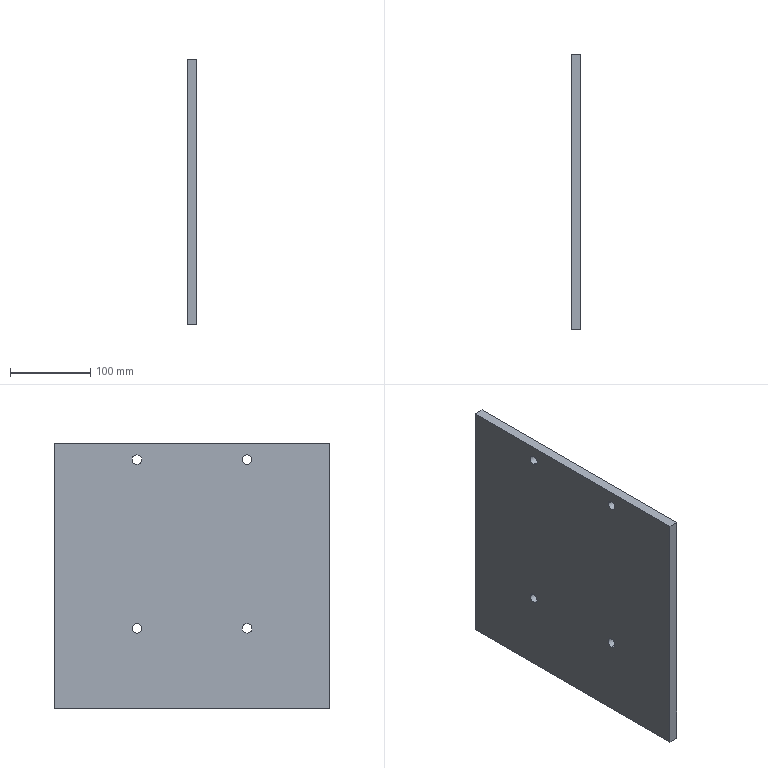Part | SolidWorks | features BaseBody 1 | 1 solid | 14 faces | box 12 x 344.147 x 330 mm | volume 1357393 mm3 | cylinder 8 | plane 6 | commonest cylinder face diameters 12 x8
STEP:
#1=CARTESIAN_POINT('',(-546.442,569.924,584.465));
#2=VERTEX_POINT('',#1);
#3=CARTESIAN_POINT('',(-546.442,569.924,596.465));
#4=VERTEX_POINT('',#3);
#5=CARTESIAN_POINT('',(-546.442,569.924,590.465));
#6=DIRECTION('',(-1.,0.,0.));
#7=DIRECTION('',(0.,0.,1.));
#8=AXIS2_PLACEMENT_3D('',#5,#6,#7);
#9=CIRCLE('',#8,6.);
#10=EDGE_CURVE('',#2,#4,#9,.T.);
#11=ORIENTED_EDGE('',*,*,#10,.T.);
#12=CARTESIAN_POINT('',(-534.442,569.924,596.465));
#13=VERTEX_POINT('',#12);
#14=CARTESIAN_POINT('',(-619.405,569.924,596.465));
#15=DIRECTION('',(1.,0.,0.));
#16=VECTOR('',#15,1000.);
#17=LINE('',#14,#16);
#18=EDGE_CURVE('',#4,#13,#17,.T.);
#19=ORIENTED_EDGE('',*,*,#18,.T.);
#20=CARTESIAN_POINT('',(-534.442,569.924,584.465));
#21=VERTEX_POINT('',#20);
#22=CARTESIAN_POINT('',(-534.442,569.924,590.465));
#23=DIRECTION('',(-1.,0.,0.));
#24=DIRECTION('',(0.,0.,1.));
#25=AXIS2_PLACEMENT_3D('',#22,#23,#24);
#26=CIRCLE('',#25,6.);
#27=EDGE_CURVE('',#21,#13,#26,.T.);
#28=ORIENTED_EDGE('',*,*,#27,.F.);
#29=CARTESIAN_POINT('',(-619.405,569.924,584.465));
#30=DIRECTION('',(1.,0.,0.));
#31=VECTOR('',#30,1000.);
#32=LINE('',#29,#31);
#33=EDGE_CURVE('',#2,#21,#32,.T.);
#34=ORIENTED_EDGE('',*,*,#33,.F.);
#35=EDGE_LOOP('',(#11,#19,#28,#34));
#36=FACE_OUTER_BOUND('',#35,.T.);
#37=CARTESIAN_POINT('',(-619.405,569.924,590.465));
#38=DIRECTION('',(1.,0.,0.));
#39=DIRECTION('',(0.,0.,-1.));
#40=AXIS2_PLACEMENT_3D('',#37,#38,#39);
#41=CYLINDRICAL_SURFACE('',#40,6.);
#42=ADVANCED_FACE('',(#36),#41,.F.);
#43=CARTESIAN_POINT('',(-546.442,569.924,590.465));
#44=DIRECTION('',(-1.,0.,0.));
#45=DIRECTION('',(0.,0.,1.));
#46=AXIS2_PLACEMENT_3D('',#43,#44,#45);
#47=CIRCLE('',#46,6.);
#48=EDGE_CURVE('',#4,#2,#47,.T.);
#49=ORIENTED_EDGE('',*,*,#48,.T.);
#50=ORIENTED_EDGE('',*,*,#33,.T.);
#51=CARTESIAN_POINT('',(-534.442,569.924,590.465));
#52=DIRECTION('',(-1.,0.,0.));
#53=DIRECTION('',(0.,0.,1.));
#54=AXIS2_PLACEMENT_3D('',#51,#52,#53);
#55=CIRCLE('',#54,6.);
#56=EDGE_CURVE('',#13,#21,#55,.T.);
#57=ORIENTED_EDGE('',*,*,#56,.F.);
#58=ORIENTED_EDGE('',*,*,#18,.F.);
#59=EDGE_LOOP('',(#49,#50,#57,#58));
#60=FACE_OUTER_BOUND('',#59,.T.);
#61=CARTESIAN_POINT('',(-619.405,569.924,590.465));
#62=DIRECTION('',(1.,0.,0.));
#63=DIRECTION('',(0.,0.,-1.));
#64=AXIS2_PLACEMENT_3D('',#61,#62,#63);
#65=CYLINDRICAL_SURFACE('',#64,6.);
#66=ADVANCED_FACE('',(#60),#65,.F.);
#67=CARTESIAN_POINT('',(-546.442,563.924,379.749));
#68=VERTEX_POINT('',#67);
#69=CARTESIAN_POINT('',(-546.442,575.924,379.749));
#70=VERTEX_POINT('',#69);
#71=CARTESIAN_POINT('',(-546.442,569.924,379.749));
#72=DIRECTION('',(-1.,0.,0.));
#73=DIRECTION('',(0.,0.,1.));
#74=AXIS2_PLACEMENT_3D('',#71,#72,#73);
#75=CIRCLE('',#74,6.);
#76=EDGE_CURVE('',#68,#70,#75,.T.);
#77=ORIENTED_EDGE('',*,*,#76,.T.);
#78=CARTESIAN_POINT('',(-534.442,575.924,379.749));
#79=VERTEX_POINT('',#78);
#80=CARTESIAN_POINT('',(-619.405,575.924,379.749));
#81=DIRECTION('',(1.,0.,0.));
#82=VECTOR('',#81,1000.);
#83=LINE('',#80,#82);
#84=EDGE_CURVE('',#70,#79,#83,.T.);
#85=ORIENTED_EDGE('',*,*,#84,.T.);
#86=CARTESIAN_POINT('',(-534.442,563.924,379.749));
#87=VERTEX_POINT('',#86);
#88=CARTESIAN_POINT('',(-534.442,569.924,379.749));
#89=DIRECTION('',(-1.,0.,0.));
#90=DIRECTION('',(0.,0.,1.));
#91=AXIS2_PLACEMENT_3D('',#88,#89,#90);
#92=CIRCLE('',#91,6.);
#93=EDGE_CURVE('',#87,#79,#92,.T.);
#94=ORIENTED_EDGE('',*,*,#93,.F.);
#95=CARTESIAN_POINT('',(-619.405,563.924,379.749));
#96=DIRECTION('',(1.,0.,0.));
#97=VECTOR('',#96,1000.);
#98=LINE('',#95,#97);
#99=EDGE_CURVE('',#68,#87,#98,.T.);
#100=ORIENTED_EDGE('',*,*,#99,.F.);
#101=EDGE_LOOP('',(#77,#85,#94,#100));
#102=FACE_OUTER_BOUND('',#101,.T.);
#103=CARTESIAN_POINT('',(-619.405,569.924,379.749));
#104=DIRECTION('',(1.,0.,0.));
#105=DIRECTION('',(0.,-1.,0.));
#106=AXIS2_PLACEMENT_3D('',#103,#104,#105);
#107=CYLINDRICAL_SURFACE('',#106,6.);
#108=ADVANCED_FACE('',(#102),#107,.F.);
#109=CARTESIAN_POINT('',(-546.442,569.924,379.749));
#110=DIRECTION('',(-1.,0.,0.));
#111=DIRECTION('',(0.,0.,1.));
#112=AXIS2_PLACEMENT_3D('',#109,#110,#111);
#113=CIRCLE('',#112,6.);
#114=EDGE_CURVE('',#70,#68,#113,.T.);
#115=ORIENTED_EDGE('',*,*,#114,.T.);
#116=ORIENTED_EDGE('',*,*,#99,.T.);
#117=CARTESIAN_POINT('',(-534.442,569.924,379.749));
#118=DIRECTION('',(-1.,0.,0.));
#119=DIRECTION('',(0.,0.,1.));
#120=AXIS2_PLACEMENT_3D('',#117,#118,#119);
#121=CIRCLE('',#120,6.);
#122=EDGE_CURVE('',#79,#87,#121,.T.);
#123=ORIENTED_EDGE('',*,*,#122,.F.);
#124=ORIENTED_EDGE('',*,*,#84,.F.);
#125=EDGE_LOOP('',(#115,#116,#123,#124));
#126=FACE_OUTER_BOUND('',#125,.T.);
#127=CARTESIAN_POINT('',(-619.405,569.924,379.749));
#128=DIRECTION('',(1.,0.,0.));
#129=DIRECTION('',(0.,-1.,0.));
#130=AXIS2_PLACEMENT_3D('',#127,#128,#129);
#131=CYLINDRICAL_SURFACE('',#130,6.);
#132=ADVANCED_FACE('',(#126),#131,.F.);
#133=CARTESIAN_POINT('',(-546.442,432.283,373.749));
#134=VERTEX_POINT('',#133);
#135=CARTESIAN_POINT('',(-546.442,432.283,385.749));
#136=VERTEX_POINT('',#135);
#137=CARTESIAN_POINT('',(-546.442,432.283,379.749));
#138=DIRECTION('',(-1.,0.,0.));
#139=DIRECTION('',(0.,0.,1.));
#140=AXIS2_PLACEMENT_3D('',#137,#138,#139);
#141=CIRCLE('',#140,6.);
#142=EDGE_CURVE('',#134,#136,#141,.T.);
#143=ORIENTED_EDGE('',*,*,#142,.T.);
#144=CARTESIAN_POINT('',(-534.442,432.283,385.749));
#145=VERTEX_POINT('',#144);
#146=CARTESIAN_POINT('',(-619.405,432.283,385.749));
#147=DIRECTION('',(1.,0.,0.));
#148=VECTOR('',#147,1000.);
#149=LINE('',#146,#148);
#150=EDGE_CURVE('',#136,#145,#149,.T.);
#151=ORIENTED_EDGE('',*,*,#150,.T.);
#152=CARTESIAN_POINT('',(-534.442,432.283,373.749));
#153=VERTEX_POINT('',#152);
#154=CARTESIAN_POINT('',(-534.442,432.283,379.749));
#155=DIRECTION('',(-1.,0.,0.));
#156=DIRECTION('',(0.,0.,1.));
#157=AXIS2_PLACEMENT_3D('',#154,#155,#156);
#158=CIRCLE('',#157,6.);
#159=EDGE_CURVE('',#153,#145,#158,.T.);
#160=ORIENTED_EDGE('',*,*,#159,.F.);
#161=CARTESIAN_POINT('',(-619.405,432.283,373.749));
#162=DIRECTION('',(1.,0.,0.));
#163=VECTOR('',#162,1000.);
#164=LINE('',#161,#163);
#165=EDGE_CURVE('',#134,#153,#164,.T.);
#166=ORIENTED_EDGE('',*,*,#165,.F.);
#167=EDGE_LOOP('',(#143,#151,#160,#166));
#168=FACE_OUTER_BOUND('',#167,.T.);
#169=CARTESIAN_POINT('',(-619.405,432.283,379.749));
#170=DIRECTION('',(1.,0.,0.));
#171=DIRECTION('',(0.,0.,-1.));
#172=AXIS2_PLACEMENT_3D('',#169,#170,#171);
#173=CYLINDRICAL_SURFACE('',#172,6.);
#174=ADVANCED_FACE('',(#168),#173,.F.);
#175=CARTESIAN_POINT('',(-546.442,432.283,379.749));
#176=DIRECTION('',(-1.,0.,0.));
#177=DIRECTION('',(0.,0.,1.));
#178=AXIS2_PLACEMENT_3D('',#175,#176,#177);
#179=CIRCLE('',#178,6.);
#180=EDGE_CURVE('',#136,#134,#179,.T.);
#181=ORIENTED_EDGE('',*,*,#180,.T.);
#182=ORIENTED_EDGE('',*,*,#165,.T.);
#183=CARTESIAN_POINT('',(-534.442,432.283,379.749));
#184=DIRECTION('',(-1.,0.,0.));
#185=DIRECTION('',(0.,0.,1.));
#186=AXIS2_PLACEMENT_3D('',#183,#184,#185);
#187=CIRCLE('',#186,6.);
#188=EDGE_CURVE('',#145,#153,#187,.T.);
#189=ORIENTED_EDGE('',*,*,#188,.F.);
#190=ORIENTED_EDGE('',*,*,#150,.F.);
#191=EDGE_LOOP('',(#181,#182,#189,#190));
#192=FACE_OUTER_BOUND('',#191,.T.);
#193=CARTESIAN_POINT('',(-619.405,432.283,379.749));
#194=DIRECTION('',(1.,0.,0.));
#195=DIRECTION('',(0.,0.,-1.));
#196=AXIS2_PLACEMENT_3D('',#193,#194,#195);
#197=CYLINDRICAL_SURFACE('',#196,6.);
#198=ADVANCED_FACE('',(#192),#197,.F.);
#199=CARTESIAN_POINT('',(-546.442,438.283,590.465));
#200=VERTEX_POINT('',#199);
#201=CARTESIAN_POINT('',(-546.442,426.283,590.465));
#202=VERTEX_POINT('',#201);
#203=CARTESIAN_POINT('',(-546.442,432.283,590.465));
#204=DIRECTION('',(-1.,0.,0.));
#205=DIRECTION('',(0.,0.,1.));
#206=AXIS2_PLACEMENT_3D('',#203,#204,#205);
#207=CIRCLE('',#206,6.);
#208=EDGE_CURVE('',#200,#202,#207,.T.);
#209=ORIENTED_EDGE('',*,*,#208,.T.);
#210=CARTESIAN_POINT('',(-534.442,426.283,590.465));
#211=VERTEX_POINT('',#210);
#212=CARTESIAN_POINT('',(-619.405,426.283,590.465));
#213=DIRECTION('',(1.,0.,0.));
#214=VECTOR('',#213,1000.);
#215=LINE('',#212,#214);
#216=EDGE_CURVE('',#202,#211,#215,.T.);
#217=ORIENTED_EDGE('',*,*,#216,.T.);
#218=CARTESIAN_POINT('',(-534.442,438.283,590.465));
#219=VERTEX_POINT('',#218);
#220=CARTESIAN_POINT('',(-534.442,432.283,590.465));
#221=DIRECTION('',(-1.,0.,0.));
#222=DIRECTION('',(0.,0.,1.));
#223=AXIS2_PLACEMENT_3D('',#220,#221,#222);
#224=CIRCLE('',#223,6.);
#225=EDGE_CURVE('',#219,#211,#224,.T.);
#226=ORIENTED_EDGE('',*,*,#225,.F.);
#227=CARTESIAN_POINT('',(-619.405,438.283,590.465));
#228=DIRECTION('',(1.,0.,0.));
#229=VECTOR('',#228,1000.);
#230=LINE('',#227,#229);
#231=EDGE_CURVE('',#200,#219,#230,.T.);
#232=ORIENTED_EDGE('',*,*,#231,.F.);
#233=EDGE_LOOP('',(#209,#217,#226,#232));
#234=FACE_OUTER_BOUND('',#233,.T.);
#235=CARTESIAN_POINT('',(-619.405,432.283,590.465));
#236=DIRECTION('',(1.,0.,0.));
#237=DIRECTION('',(0.,1.,0.));
#238=AXIS2_PLACEMENT_3D('',#235,#236,#237);
#239=CYLINDRICAL_SURFACE('',#238,6.);
#240=ADVANCED_FACE('',(#234),#239,.F.);
#241=CARTESIAN_POINT('',(-546.442,432.283,590.465));
#242=DIRECTION('',(-1.,0.,0.));
#243=DIRECTION('',(0.,0.,1.));
#244=AXIS2_PLACEMENT_3D('',#241,#242,#243);
#245=CIRCLE('',#244,6.);
#246=EDGE_CURVE('',#202,#200,#245,.T.);
#247=ORIENTED_EDGE('',*,*,#246,.T.);
#248=ORIENTED_EDGE('',*,*,#231,.T.);
#249=CARTESIAN_POINT('',(-534.442,432.283,590.465));
#250=DIRECTION('',(-1.,0.,0.));
#251=DIRECTION('',(0.,0.,1.));
#252=AXIS2_PLACEMENT_3D('',#249,#250,#251);
#253=CIRCLE('',#252,6.);
#254=EDGE_CURVE('',#211,#219,#253,.T.);
#255=ORIENTED_EDGE('',*,*,#254,.F.);
#256=ORIENTED_EDGE('',*,*,#216,.F.);
#257=EDGE_LOOP('',(#247,#248,#255,#256));
#258=FACE_OUTER_BOUND('',#257,.T.);
#259=CARTESIAN_POINT('',(-619.405,432.283,590.465));
#260=DIRECTION('',(1.,0.,0.));
#261=DIRECTION('',(0.,1.,0.));
#262=AXIS2_PLACEMENT_3D('',#259,#260,#261);
#263=CYLINDRICAL_SURFACE('',#262,6.);
#264=ADVANCED_FACE('',(#258),#263,.F.);
#265=ORIENTED_EDGE('',*,*,#225,.T.);
#266=ORIENTED_EDGE('',*,*,#254,.T.);
#267=EDGE_LOOP('',(#265,#266));
#268=FACE_BOUND('',#267,.T.);
#269=ORIENTED_EDGE('',*,*,#159,.T.);
#270=ORIENTED_EDGE('',*,*,#188,.T.);
#271=EDGE_LOOP('',(#269,#270));
#272=FACE_BOUND('',#271,.T.);
#273=ORIENTED_EDGE('',*,*,#93,.T.);
#274=ORIENTED_EDGE('',*,*,#122,.T.);
#275=EDGE_LOOP('',(#273,#274));
#276=FACE_BOUND('',#275,.T.);
#277=ORIENTED_EDGE('',*,*,#27,.T.);
#278=ORIENTED_EDGE('',*,*,#56,.T.);
#279=EDGE_LOOP('',(#277,#278));
#280=FACE_BOUND('',#279,.T.);
#281=CARTESIAN_POINT('',(-534.442,329.03,280.107));
#282=VERTEX_POINT('',#281);
#283=CARTESIAN_POINT('',(-534.442,673.177,280.107));
#284=VERTEX_POINT('',#283);
#285=CARTESIAN_POINT('',(-534.442,409.03,280.107));
#286=DIRECTION('',(0.,1.,0.));
#287=VECTOR('',#286,1000.);
#288=LINE('',#285,#287);
#289=EDGE_CURVE('',#282,#284,#288,.T.);
#290=ORIENTED_EDGE('',*,*,#289,.T.);
#291=CARTESIAN_POINT('',(-534.442,673.177,610.107));
#292=VERTEX_POINT('',#291);
#293=CARTESIAN_POINT('',(-534.442,673.177,610.107));
#294=DIRECTION('',(0.,0.,1.));
#295=VECTOR('',#294,1000.);
#296=LINE('',#293,#295);
#297=EDGE_CURVE('',#284,#292,#296,.T.);
#298=ORIENTED_EDGE('',*,*,#297,.T.);
#299=CARTESIAN_POINT('',(-534.442,329.03,610.107));
#300=VERTEX_POINT('',#299);
#301=CARTESIAN_POINT('',(-534.442,409.03,610.107));
#302=DIRECTION('',(0.,-1.,0.));
#303=VECTOR('',#302,1000.);
#304=LINE('',#301,#303);
#305=EDGE_CURVE('',#292,#300,#304,.T.);
#306=ORIENTED_EDGE('',*,*,#305,.T.);
#307=CARTESIAN_POINT('',(-534.442,329.03,610.107));
#308=DIRECTION('',(0.,0.,-1.));
#309=VECTOR('',#308,1000.);
#310=LINE('',#307,#309);
#311=EDGE_CURVE('',#300,#282,#310,.T.);
#312=ORIENTED_EDGE('',*,*,#311,.T.);
#313=EDGE_LOOP('',(#290,#298,#306,#312));
#314=FACE_OUTER_BOUND('',#313,.T.);
#315=CARTESIAN_POINT('',(-534.442,409.03,610.107));
#316=DIRECTION('',(-1.,0.,0.));
#317=DIRECTION('',(0.,0.,1.));
#318=AXIS2_PLACEMENT_3D('',#315,#316,#317);
#319=PLANE('',#318);
#320=ADVANCED_FACE('',(#268,#272,#276,#280,#314),#319,.F.);
#321=CARTESIAN_POINT('',(-546.442,673.177,280.107));
#322=VERTEX_POINT('',#321);
#323=CARTESIAN_POINT('',(-546.442,329.03,280.107));
#324=VERTEX_POINT('',#323);
#325=CARTESIAN_POINT('',(-546.442,593.177,280.107));
#326=DIRECTION('',(0.,-1.,0.));
#327=VECTOR('',#326,1000.);
#328=LINE('',#325,#327);
#329=EDGE_CURVE('',#322,#324,#328,.T.);
#330=ORIENTED_EDGE('',*,*,#329,.F.);
#331=CARTESIAN_POINT('',(-546.442,673.177,280.107));
#332=DIRECTION('',(1.,0.,0.));
#333=VECTOR('',#332,1000.);
#334=LINE('',#331,#333);
#335=EDGE_CURVE('',#322,#284,#334,.T.);
#336=ORIENTED_EDGE('',*,*,#335,.T.);
#337=ORIENTED_EDGE('',*,*,#289,.F.);
#338=CARTESIAN_POINT('',(-546.442,329.03,280.107));
#339=DIRECTION('',(-1.,0.,0.));
#340=VECTOR('',#339,1000.);
#341=LINE('',#338,#340);
#342=EDGE_CURVE('',#282,#324,#341,.T.);
#343=ORIENTED_EDGE('',*,*,#342,.T.);
#344=EDGE_LOOP('',(#330,#336,#337,#343));
#345=FACE_OUTER_BOUND('',#344,.T.);
#346=CARTESIAN_POINT('',(-546.442,593.177,280.107));
#347=DIRECTION('',(0.,0.,1.));
#348=DIRECTION('',(0.,-1.,0.));
#349=AXIS2_PLACEMENT_3D('',#346,#347,#348);
#350=PLANE('',#349);
#351=ADVANCED_FACE('',(#345),#350,.F.);
#352=CARTESIAN_POINT('',(-546.442,329.03,610.107));
#353=VERTEX_POINT('',#352);
#354=CARTESIAN_POINT('',(-546.442,329.03,360.107));
#355=DIRECTION('',(0.,0.,1.));
#356=VECTOR('',#355,1000.);
#357=LINE('',#354,#356);
#358=EDGE_CURVE('',#324,#353,#357,.T.);
#359=ORIENTED_EDGE('',*,*,#358,.F.);
#360=ORIENTED_EDGE('',*,*,#342,.F.);
#361=ORIENTED_EDGE('',*,*,#311,.F.);
#362=CARTESIAN_POINT('',(-546.442,329.03,610.107));
#363=DIRECTION('',(-1.,0.,0.));
#364=VECTOR('',#363,1000.);
#365=LINE('',#362,#364);
#366=EDGE_CURVE('',#300,#353,#365,.T.);
#367=ORIENTED_EDGE('',*,*,#366,.T.);
#368=EDGE_LOOP('',(#359,#360,#361,#367));
#369=FACE_OUTER_BOUND('',#368,.T.);
#370=CARTESIAN_POINT('',(-546.442,329.03,360.107));
#371=DIRECTION('',(0.,1.,0.));
#372=DIRECTION('',(1.,0.,0.));
#373=AXIS2_PLACEMENT_3D('',#370,#371,#372);
#374=PLANE('',#373);
#375=ADVANCED_FACE('',(#369),#374,.F.);
#376=CARTESIAN_POINT('',(-546.442,673.177,610.107));
#377=VERTEX_POINT('',#376);
#378=CARTESIAN_POINT('',(-546.442,409.03,610.107));
#379=DIRECTION('',(0.,1.,0.));
#380=VECTOR('',#379,1000.);
#381=LINE('',#378,#380);
#382=EDGE_CURVE('',#353,#377,#381,.T.);
#383=ORIENTED_EDGE('',*,*,#382,.F.);
#384=ORIENTED_EDGE('',*,*,#366,.F.);
#385=ORIENTED_EDGE('',*,*,#305,.F.);
#386=CARTESIAN_POINT('',(-546.442,673.177,610.107));
#387=DIRECTION('',(-1.,0.,0.));
#388=VECTOR('',#387,1000.);
#389=LINE('',#386,#388);
#390=EDGE_CURVE('',#292,#377,#389,.T.);
#391=ORIENTED_EDGE('',*,*,#390,.T.);
#392=EDGE_LOOP('',(#383,#384,#385,#391));
#393=FACE_OUTER_BOUND('',#392,.T.);
#394=CARTESIAN_POINT('',(-546.442,409.03,610.107));
#395=DIRECTION('',(0.,0.,-1.));
#396=DIRECTION('',(0.,-1.,0.));
#397=AXIS2_PLACEMENT_3D('',#394,#395,#396);
#398=PLANE('',#397);
#399=ADVANCED_FACE('',(#393),#398,.F.);
#400=CARTESIAN_POINT('',(-546.442,673.177,610.107));
#401=DIRECTION('',(0.,0.,-1.));
#402=VECTOR('',#401,1000.);
#403=LINE('',#400,#402);
#404=EDGE_CURVE('',#377,#322,#403,.T.);
#405=ORIENTED_EDGE('',*,*,#404,.F.);
#406=ORIENTED_EDGE('',*,*,#390,.F.);
#407=ORIENTED_EDGE('',*,*,#297,.F.);
#408=ORIENTED_EDGE('',*,*,#335,.F.);
#409=EDGE_LOOP('',(#405,#406,#407,#408));
#410=FACE_OUTER_BOUND('',#409,.T.);
#411=CARTESIAN_POINT('',(-546.442,673.177,610.107));
#412=DIRECTION('',(0.,-1.,0.));
#413=DIRECTION('',(0.,0.,-1.));
#414=AXIS2_PLACEMENT_3D('',#411,#412,#413);
#415=PLANE('',#414);
#416=ADVANCED_FACE('',(#410),#415,.F.);
#417=ORIENTED_EDGE('',*,*,#246,.F.);
#418=ORIENTED_EDGE('',*,*,#208,.F.);
#419=EDGE_LOOP('',(#417,#418));
#420=FACE_BOUND('',#419,.T.);
#421=ORIENTED_EDGE('',*,*,#180,.F.);
#422=ORIENTED_EDGE('',*,*,#142,.F.);
#423=EDGE_LOOP('',(#421,#422));
#424=FACE_BOUND('',#423,.T.);
#425=ORIENTED_EDGE('',*,*,#114,.F.);
#426=ORIENTED_EDGE('',*,*,#76,.F.);
#427=EDGE_LOOP('',(#425,#426));
#428=FACE_BOUND('',#427,.T.);
#429=ORIENTED_EDGE('',*,*,#48,.F.);
#430=ORIENTED_EDGE('',*,*,#10,.F.);
#431=EDGE_LOOP('',(#429,#430));
#432=FACE_BOUND('',#431,.T.);
#433=ORIENTED_EDGE('',*,*,#382,.T.);
#434=ORIENTED_EDGE('',*,*,#404,.T.);
#435=ORIENTED_EDGE('',*,*,#329,.T.);
#436=ORIENTED_EDGE('',*,*,#358,.T.);
#437=EDGE_LOOP('',(#433,#434,#435,#436));
#438=FACE_OUTER_BOUND('',#437,.T.);
#439=CARTESIAN_POINT('',(-546.442,409.03,610.107));
#440=DIRECTION('',(-1.,0.,0.));
#441=DIRECTION('',(0.,0.,1.));
#442=AXIS2_PLACEMENT_3D('',#439,#440,#441);
#443=PLANE('',#442);
#444=ADVANCED_FACE('',(#420,#424,#428,#432,#438),#443,.T.);
#445=CLOSED_SHELL('',(#42,#66,#108,#132,#174,#198,#240,#264,#320,#351,#375,#399,#416,#444));
#446=MANIFOLD_SOLID_BREP('',#445);
#447=CARTESIAN_POINT('',(0.,0.,0.));
#448=DIRECTION('',(0.,0.,1.));
#449=DIRECTION('',(1.,0.,0.));
#450=AXIS2_PLACEMENT_3D('',#447,#448,#449);
#451=(LENGTH_UNIT()NAMED_UNIT(*)SI_UNIT(.MILLI.,.METRE.));
#452=UNCERTAINTY_MEASURE_WITH_UNIT(LENGTH_MEASURE(0.00001),#451,'','');
#453=(NAMED_UNIT(*)PLANE_ANGLE_UNIT()SI_UNIT($,.RADIAN.));
#454=(NAMED_UNIT(*)SI_UNIT($,.STERADIAN.)SOLID_ANGLE_UNIT());
#455=(GEOMETRIC_REPRESENTATION_CONTEXT(3)GLOBAL_UNCERTAINTY_ASSIGNED_CONTEXT((#452))GLOBAL_UNIT_ASSIGNED_CONTEXT((#451,#453,#454))REPRESENTATION_CONTEXT('',''));
#456=ADVANCED_BREP_SHAPE_REPRESENTATION('',(#446,#450),#455);